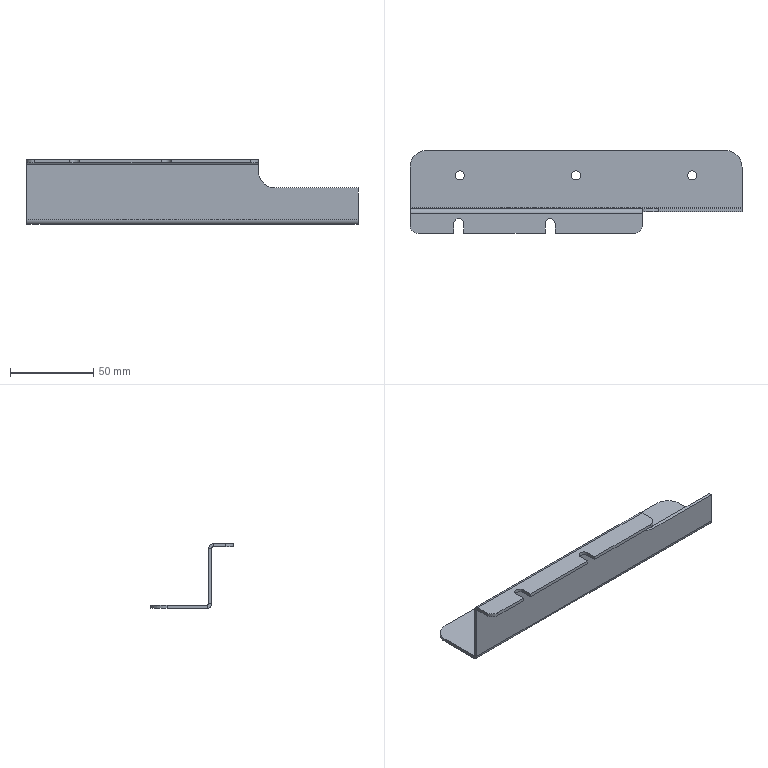Part | STEP file | 09-36 left support plate (Default) | 1 solid | 43 faces | box 200 x 50 x 39 mm | volume 30286 mm3 | plane 26 | cylinder 17 | commonest cylinder face diameters 5.5 x6 20 x3 1.473 x2 5.473 x2 6 x2 10 x2
STEP:
#1=CARTESIAN_POINT('',(-72.75,2.5,0.));
#2=VERTEX_POINT('',#1);
#3=CARTESIAN_POINT('',(-67.25,2.5,0.));
#4=VERTEX_POINT('',#3);
#5=CARTESIAN_POINT('',(-70.,2.5,0.));
#6=DIRECTION('',(0.,0.,1.));
#7=DIRECTION('',(1.,0.,0.));
#8=AXIS2_PLACEMENT_3D('',#5,#6,#7);
#9=CIRCLE('',#8,2.75);
#10=EDGE_CURVE('',#2,#4,#9,.T.);
#11=ORIENTED_EDGE('',*,*,#10,.T.);
#12=CARTESIAN_POINT('',(-67.25,2.5,-2.));
#13=VERTEX_POINT('',#12);
#14=CARTESIAN_POINT('',(-67.25,2.5,28.));
#15=DIRECTION('',(0.,0.,-1.));
#16=VECTOR('',#15,1000.);
#17=LINE('',#14,#16);
#18=EDGE_CURVE('',#4,#13,#17,.T.);
#19=ORIENTED_EDGE('',*,*,#18,.T.);
#20=CARTESIAN_POINT('',(-72.75,2.5,-2.));
#21=VERTEX_POINT('',#20);
#22=CARTESIAN_POINT('',(-70.,2.5,-2.));
#23=DIRECTION('',(0.,0.,-1.));
#24=DIRECTION('',(-1.,0.,0.));
#25=AXIS2_PLACEMENT_3D('',#22,#23,#24);
#26=CIRCLE('',#25,2.75);
#27=EDGE_CURVE('',#13,#21,#26,.T.);
#28=ORIENTED_EDGE('',*,*,#27,.T.);
#29=CARTESIAN_POINT('',(-72.75,2.5,28.));
#30=DIRECTION('',(0.,0.,-1.));
#31=VECTOR('',#30,1000.);
#32=LINE('',#29,#31);
#33=EDGE_CURVE('',#2,#21,#32,.T.);
#34=ORIENTED_EDGE('',*,*,#33,.F.);
#35=EDGE_LOOP('',(#11,#19,#28,#34));
#36=FACE_OUTER_BOUND('',#35,.T.);
#37=CARTESIAN_POINT('',(-70.,2.5,28.));
#38=DIRECTION('',(0.,0.,-1.));
#39=DIRECTION('',(-1.,0.,0.));
#40=AXIS2_PLACEMENT_3D('',#37,#38,#39);
#41=CYLINDRICAL_SURFACE('',#40,2.75);
#42=ADVANCED_FACE('',(#36),#41,.F.);
#43=CARTESIAN_POINT('',(-2.75,2.5,0.));
#44=VERTEX_POINT('',#43);
#45=CARTESIAN_POINT('',(2.75,2.5,0.));
#46=VERTEX_POINT('',#45);
#47=CARTESIAN_POINT('',(0.,2.5,0.));
#48=DIRECTION('',(0.,0.,1.));
#49=DIRECTION('',(1.,0.,0.));
#50=AXIS2_PLACEMENT_3D('',#47,#48,#49);
#51=CIRCLE('',#50,2.75);
#52=EDGE_CURVE('',#44,#46,#51,.T.);
#53=ORIENTED_EDGE('',*,*,#52,.T.);
#54=CARTESIAN_POINT('',(2.75,2.5,-2.));
#55=VERTEX_POINT('',#54);
#56=CARTESIAN_POINT('',(2.75,2.5,28.));
#57=DIRECTION('',(0.,0.,-1.));
#58=VECTOR('',#57,1000.);
#59=LINE('',#56,#58);
#60=EDGE_CURVE('',#46,#55,#59,.T.);
#61=ORIENTED_EDGE('',*,*,#60,.T.);
#62=CARTESIAN_POINT('',(-2.75,2.5,-2.));
#63=VERTEX_POINT('',#62);
#64=CARTESIAN_POINT('',(0.,2.5,-2.));
#65=DIRECTION('',(0.,0.,-1.));
#66=DIRECTION('',(-1.,0.,0.));
#67=AXIS2_PLACEMENT_3D('',#64,#65,#66);
#68=CIRCLE('',#67,2.75);
#69=EDGE_CURVE('',#55,#63,#68,.T.);
#70=ORIENTED_EDGE('',*,*,#69,.T.);
#71=CARTESIAN_POINT('',(-2.75,2.5,28.));
#72=DIRECTION('',(0.,0.,-1.));
#73=VECTOR('',#72,1000.);
#74=LINE('',#71,#73);
#75=EDGE_CURVE('',#44,#63,#74,.T.);
#76=ORIENTED_EDGE('',*,*,#75,.F.);
#77=EDGE_LOOP('',(#53,#61,#70,#76));
#78=FACE_OUTER_BOUND('',#77,.T.);
#79=CARTESIAN_POINT('',(0.,2.5,28.));
#80=DIRECTION('',(0.,0.,-1.));
#81=DIRECTION('',(-1.,0.,0.));
#82=AXIS2_PLACEMENT_3D('',#79,#80,#81);
#83=CYLINDRICAL_SURFACE('',#82,2.75);
#84=ADVANCED_FACE('',(#78),#83,.F.);
#85=CARTESIAN_POINT('',(67.25,2.5,0.));
#86=VERTEX_POINT('',#85);
#87=CARTESIAN_POINT('',(72.75,2.5,0.));
#88=VERTEX_POINT('',#87);
#89=CARTESIAN_POINT('',(70.,2.5,0.));
#90=DIRECTION('',(0.,0.,1.));
#91=DIRECTION('',(1.,0.,0.));
#92=AXIS2_PLACEMENT_3D('',#89,#90,#91);
#93=CIRCLE('',#92,2.75);
#94=EDGE_CURVE('',#86,#88,#93,.T.);
#95=ORIENTED_EDGE('',*,*,#94,.T.);
#96=CARTESIAN_POINT('',(72.75,2.5,-2.));
#97=VERTEX_POINT('',#96);
#98=CARTESIAN_POINT('',(72.75,2.5,28.));
#99=DIRECTION('',(0.,0.,-1.));
#100=VECTOR('',#99,1000.);
#101=LINE('',#98,#100);
#102=EDGE_CURVE('',#88,#97,#101,.T.);
#103=ORIENTED_EDGE('',*,*,#102,.T.);
#104=CARTESIAN_POINT('',(67.25,2.5,-2.));
#105=VERTEX_POINT('',#104);
#106=CARTESIAN_POINT('',(70.,2.5,-2.));
#107=DIRECTION('',(0.,0.,-1.));
#108=DIRECTION('',(-1.,0.,0.));
#109=AXIS2_PLACEMENT_3D('',#106,#107,#108);
#110=CIRCLE('',#109,2.75);
#111=EDGE_CURVE('',#97,#105,#110,.T.);
#112=ORIENTED_EDGE('',*,*,#111,.T.);
#113=CARTESIAN_POINT('',(67.25,2.5,28.));
#114=DIRECTION('',(0.,0.,-1.));
#115=VECTOR('',#114,1000.);
#116=LINE('',#113,#115);
#117=EDGE_CURVE('',#86,#105,#116,.T.);
#118=ORIENTED_EDGE('',*,*,#117,.F.);
#119=EDGE_LOOP('',(#95,#103,#112,#118));
#120=FACE_OUTER_BOUND('',#119,.T.);
#121=CARTESIAN_POINT('',(70.,2.5,28.));
#122=DIRECTION('',(0.,0.,-1.));
#123=DIRECTION('',(-1.,0.,0.));
#124=AXIS2_PLACEMENT_3D('',#121,#122,#123);
#125=CYLINDRICAL_SURFACE('',#124,2.75);
#126=ADVANCED_FACE('',(#120),#125,.F.);
#127=CARTESIAN_POINT('',(-12.6,-32.5,35.));
#128=VERTEX_POINT('',#127);
#129=CARTESIAN_POINT('',(-12.6,-32.5,37.));
#130=VERTEX_POINT('',#129);
#131=CARTESIAN_POINT('',(-12.6,-32.5,7.));
#132=DIRECTION('',(0.,0.,1.));
#133=VECTOR('',#132,1000.);
#134=LINE('',#131,#133);
#135=EDGE_CURVE('',#128,#130,#134,.T.);
#136=ORIENTED_EDGE('',*,*,#135,.F.);
#137=CARTESIAN_POINT('',(35.,-32.5,35.));
#138=VERTEX_POINT('',#137);
#139=CARTESIAN_POINT('',(-100.,-32.5,35.));
#140=DIRECTION('',(-1.,0.,0.));
#141=VECTOR('',#140,1000.);
#142=LINE('',#139,#141);
#143=EDGE_CURVE('',#138,#128,#142,.T.);
#144=ORIENTED_EDGE('',*,*,#143,.F.);
#145=CARTESIAN_POINT('',(35.,-32.5,37.));
#146=VERTEX_POINT('',#145);
#147=CARTESIAN_POINT('',(35.,-32.5,37.));
#148=DIRECTION('',(0.,0.,1.));
#149=VECTOR('',#148,1000.);
#150=LINE('',#147,#149);
#151=EDGE_CURVE('',#138,#146,#150,.T.);
#152=ORIENTED_EDGE('',*,*,#151,.T.);
#153=CARTESIAN_POINT('',(-100.,-32.5,37.));
#154=DIRECTION('',(-1.,0.,0.));
#155=VECTOR('',#154,1000.);
#156=LINE('',#153,#155);
#157=EDGE_CURVE('',#146,#130,#156,.T.);
#158=ORIENTED_EDGE('',*,*,#157,.T.);
#159=EDGE_LOOP('',(#136,#144,#152,#158));
#160=FACE_OUTER_BOUND('',#159,.T.);
#161=CARTESIAN_POINT('',(-100.,-32.5,37.));
#162=DIRECTION('',(0.,-1.,0.));
#163=DIRECTION('',(0.,0.,-1.));
#164=AXIS2_PLACEMENT_3D('',#161,#162,#163);
#165=PLANE('',#164);
#166=ADVANCED_FACE('',(#160),#165,.T.);
#167=CARTESIAN_POINT('',(-18.6,-32.5,35.));
#168=VERTEX_POINT('',#167);
#169=CARTESIAN_POINT('',(-18.6,-32.5,37.));
#170=VERTEX_POINT('',#169);
#171=CARTESIAN_POINT('',(-18.6,-32.5,7.));
#172=DIRECTION('',(0.,0.,1.));
#173=VECTOR('',#172,1000.);
#174=LINE('',#171,#173);
#175=EDGE_CURVE('',#168,#170,#174,.T.);
#176=ORIENTED_EDGE('',*,*,#175,.T.);
#177=CARTESIAN_POINT('',(-67.6,-32.5,37.));
#178=VERTEX_POINT('',#177);
#179=CARTESIAN_POINT('',(-100.,-32.5,37.));
#180=DIRECTION('',(-1.,0.,0.));
#181=VECTOR('',#180,1000.);
#182=LINE('',#179,#181);
#183=EDGE_CURVE('',#170,#178,#182,.T.);
#184=ORIENTED_EDGE('',*,*,#183,.T.);
#185=CARTESIAN_POINT('',(-67.6,-32.5,35.));
#186=VERTEX_POINT('',#185);
#187=CARTESIAN_POINT('',(-67.6,-32.5,7.));
#188=DIRECTION('',(0.,0.,1.));
#189=VECTOR('',#188,1000.);
#190=LINE('',#187,#189);
#191=EDGE_CURVE('',#186,#178,#190,.T.);
#192=ORIENTED_EDGE('',*,*,#191,.F.);
#193=CARTESIAN_POINT('',(-100.,-32.5,35.));
#194=DIRECTION('',(-1.,0.,0.));
#195=VECTOR('',#194,1000.);
#196=LINE('',#193,#195);
#197=EDGE_CURVE('',#168,#186,#196,.T.);
#198=ORIENTED_EDGE('',*,*,#197,.F.);
#199=EDGE_LOOP('',(#176,#184,#192,#198));
#200=FACE_OUTER_BOUND('',#199,.T.);
#201=CARTESIAN_POINT('',(-100.,-32.5,37.));
#202=DIRECTION('',(0.,-1.,0.));
#203=DIRECTION('',(0.,0.,-1.));
#204=AXIS2_PLACEMENT_3D('',#201,#202,#203);
#205=PLANE('',#204);
#206=ADVANCED_FACE('',(#200),#205,.T.);
#207=CARTESIAN_POINT('',(100.,-19.5,20.));
#208=VERTEX_POINT('',#207);
#209=CARTESIAN_POINT('',(100.,-19.5,0.7366));
#210=VERTEX_POINT('',#209);
#211=CARTESIAN_POINT('',(100.,-19.5,0.));
#212=DIRECTION('',(0.,0.,-1.));
#213=VECTOR('',#212,1000.);
#214=LINE('',#211,#213);
#215=EDGE_CURVE('',#208,#210,#214,.T.);
#216=ORIENTED_EDGE('',*,*,#215,.F.);
#217=CARTESIAN_POINT('',(50.,-19.5,20.));
#218=VERTEX_POINT('',#217);
#219=CARTESIAN_POINT('',(100.,-19.5,20.));
#220=DIRECTION('',(-1.,0.,0.));
#221=VECTOR('',#220,1000.);
#222=LINE('',#219,#221);
#223=EDGE_CURVE('',#208,#218,#222,.T.);
#224=ORIENTED_EDGE('',*,*,#223,.T.);
#225=CARTESIAN_POINT('',(40.,-19.5,30.));
#226=VERTEX_POINT('',#225);
#227=CARTESIAN_POINT('',(50.,-19.5,30.));
#228=DIRECTION('',(0.,1.,0.));
#229=DIRECTION('',(0.,0.,1.));
#230=AXIS2_PLACEMENT_3D('',#227,#228,#229);
#231=CIRCLE('',#230,10.);
#232=EDGE_CURVE('',#218,#226,#231,.T.);
#233=ORIENTED_EDGE('',*,*,#232,.T.);
#234=CARTESIAN_POINT('',(40.,-19.5,34.263));
#235=VERTEX_POINT('',#234);
#236=CARTESIAN_POINT('',(40.,-19.5,0.));
#237=DIRECTION('',(0.,0.,1.));
#238=VECTOR('',#237,1000.);
#239=LINE('',#236,#238);
#240=EDGE_CURVE('',#226,#235,#239,.T.);
#241=ORIENTED_EDGE('',*,*,#240,.T.);
#242=CARTESIAN_POINT('',(-100.,-19.5,34.263));
#243=VERTEX_POINT('',#242);
#244=CARTESIAN_POINT('',(-100.,-19.5,34.263));
#245=DIRECTION('',(1.,0.,0.));
#246=VECTOR('',#245,1000.);
#247=LINE('',#244,#246);
#248=EDGE_CURVE('',#243,#235,#247,.T.);
#249=ORIENTED_EDGE('',*,*,#248,.F.);
#250=CARTESIAN_POINT('',(-100.,-19.5,0.7366));
#251=VERTEX_POINT('',#250);
#252=CARTESIAN_POINT('',(-100.,-19.5,35.));
#253=DIRECTION('',(0.,0.,1.));
#254=VECTOR('',#253,1000.);
#255=LINE('',#252,#254);
#256=EDGE_CURVE('',#251,#243,#255,.T.);
#257=ORIENTED_EDGE('',*,*,#256,.F.);
#258=CARTESIAN_POINT('',(100.,-19.5,0.7366));
#259=DIRECTION('',(1.,0.,0.));
#260=VECTOR('',#259,1000.);
#261=LINE('',#258,#260);
#262=EDGE_CURVE('',#251,#210,#261,.T.);
#263=ORIENTED_EDGE('',*,*,#262,.T.);
#264=EDGE_LOOP('',(#216,#224,#233,#241,#249,#257,#263));
#265=FACE_OUTER_BOUND('',#264,.T.);
#266=CARTESIAN_POINT('',(100.,-19.5,0.));
#267=DIRECTION('',(0.,-1.,0.));
#268=DIRECTION('',(0.,0.,-1.));
#269=AXIS2_PLACEMENT_3D('',#266,#267,#268);
#270=PLANE('',#269);
#271=ADVANCED_FACE('',(#265),#270,.T.);
#272=CARTESIAN_POINT('',(100.,-17.5,20.));
#273=VERTEX_POINT('',#272);
#274=CARTESIAN_POINT('',(50.,-17.5,20.));
#275=VERTEX_POINT('',#274);
#276=CARTESIAN_POINT('',(126.294,-17.5,20.));
#277=DIRECTION('',(-1.,0.,0.));
#278=VECTOR('',#277,1000.);
#279=LINE('',#276,#278);
#280=EDGE_CURVE('',#273,#275,#279,.T.);
#281=ORIENTED_EDGE('',*,*,#280,.F.);
#282=CARTESIAN_POINT('',(100.,-17.5,0.7366));
#283=VERTEX_POINT('',#282);
#284=CARTESIAN_POINT('',(100.,-17.5,0.));
#285=DIRECTION('',(0.,0.,-1.));
#286=VECTOR('',#285,1000.);
#287=LINE('',#284,#286);
#288=EDGE_CURVE('',#273,#283,#287,.T.);
#289=ORIENTED_EDGE('',*,*,#288,.T.);
#290=CARTESIAN_POINT('',(-100.,-17.5,0.7366));
#291=VERTEX_POINT('',#290);
#292=CARTESIAN_POINT('',(-100.,-17.5,0.7366));
#293=DIRECTION('',(1.,0.,0.));
#294=VECTOR('',#293,1000.);
#295=LINE('',#292,#294);
#296=EDGE_CURVE('',#291,#283,#295,.T.);
#297=ORIENTED_EDGE('',*,*,#296,.F.);
#298=CARTESIAN_POINT('',(-100.,-17.5,34.263));
#299=VERTEX_POINT('',#298);
#300=CARTESIAN_POINT('',(-100.,-17.5,35.));
#301=DIRECTION('',(0.,0.,1.));
#302=VECTOR('',#301,1000.);
#303=LINE('',#300,#302);
#304=EDGE_CURVE('',#291,#299,#303,.T.);
#305=ORIENTED_EDGE('',*,*,#304,.T.);
#306=CARTESIAN_POINT('',(40.,-17.5,34.263));
#307=VERTEX_POINT('',#306);
#308=CARTESIAN_POINT('',(-100.,-17.5,34.263));
#309=DIRECTION('',(1.,0.,0.));
#310=VECTOR('',#309,1000.);
#311=LINE('',#308,#310);
#312=EDGE_CURVE('',#299,#307,#311,.T.);
#313=ORIENTED_EDGE('',*,*,#312,.T.);
#314=CARTESIAN_POINT('',(40.,-17.5,30.));
#315=VERTEX_POINT('',#314);
#316=CARTESIAN_POINT('',(40.,-17.5,30.));
#317=DIRECTION('',(0.,0.,1.));
#318=VECTOR('',#317,1000.);
#319=LINE('',#316,#318);
#320=EDGE_CURVE('',#315,#307,#319,.T.);
#321=ORIENTED_EDGE('',*,*,#320,.F.);
#322=CARTESIAN_POINT('',(50.,-17.5,30.));
#323=DIRECTION('',(0.,1.,0.));
#324=DIRECTION('',(0.,0.,-1.));
#325=AXIS2_PLACEMENT_3D('',#322,#323,#324);
#326=CIRCLE('',#325,10.);
#327=EDGE_CURVE('',#275,#315,#326,.T.);
#328=ORIENTED_EDGE('',*,*,#327,.F.);
#329=EDGE_LOOP('',(#281,#289,#297,#305,#313,#321,#328));
#330=FACE_OUTER_BOUND('',#329,.T.);
#331=CARTESIAN_POINT('',(100.,-17.5,0.));
#332=DIRECTION('',(0.,-1.,0.));
#333=DIRECTION('',(0.,0.,-1.));
#334=AXIS2_PLACEMENT_3D('',#331,#332,#333);
#335=PLANE('',#334);
#336=ADVANCED_FACE('',(#330),#335,.F.);
#337=ORIENTED_EDGE('',*,*,#288,.F.);
#338=CARTESIAN_POINT('',(100.,-17.5,20.));
#339=DIRECTION('',(0.,-1.,0.));
#340=VECTOR('',#339,1000.);
#341=LINE('',#338,#340);
#342=EDGE_CURVE('',#273,#208,#341,.T.);
#343=ORIENTED_EDGE('',*,*,#342,.T.);
#344=ORIENTED_EDGE('',*,*,#215,.T.);
#345=CARTESIAN_POINT('',(100.,-17.5,0.7366));
#346=DIRECTION('',(0.,-1.,0.));
#347=VECTOR('',#346,1000.);
#348=LINE('',#345,#347);
#349=EDGE_CURVE('',#283,#210,#348,.T.);
#350=ORIENTED_EDGE('',*,*,#349,.F.);
#351=EDGE_LOOP('',(#337,#343,#344,#350));
#352=FACE_OUTER_BOUND('',#351,.T.);
#353=CARTESIAN_POINT('',(100.,-19.5,0.));
#354=DIRECTION('',(1.,0.,0.));
#355=DIRECTION('',(0.,0.,-1.));
#356=AXIS2_PLACEMENT_3D('',#353,#354,#355);
#357=PLANE('',#356);
#358=ADVANCED_FACE('',(#352),#357,.T.);
#359=CARTESIAN_POINT('',(40.,-20.237,37.));
#360=VERTEX_POINT('',#359);
#361=CARTESIAN_POINT('',(-100.,-20.237,37.));
#362=VERTEX_POINT('',#361);
#363=CARTESIAN_POINT('',(-100.,-20.237,37.));
#364=DIRECTION('',(-1.,0.,0.));
#365=VECTOR('',#364,1000.);
#366=LINE('',#363,#365);
#367=EDGE_CURVE('',#360,#362,#366,.T.);
#368=ORIENTED_EDGE('',*,*,#367,.F.);
#369=CARTESIAN_POINT('',(40.,-20.237,34.263));
#370=DIRECTION('',(1.,0.,0.));
#371=DIRECTION('',(0.,0.,1.));
#372=AXIS2_PLACEMENT_3D('',#369,#370,#371);
#373=CIRCLE('',#372,2.737);
#374=EDGE_CURVE('',#307,#360,#373,.T.);
#375=ORIENTED_EDGE('',*,*,#374,.F.);
#376=ORIENTED_EDGE('',*,*,#312,.F.);
#377=CARTESIAN_POINT('',(-100.,-20.237,34.263));
#378=DIRECTION('',(-1.,0.,0.));
#379=DIRECTION('',(0.,0.,1.));
#380=AXIS2_PLACEMENT_3D('',#377,#378,#379);
#381=CIRCLE('',#380,2.737);
#382=EDGE_CURVE('',#362,#299,#381,.T.);
#383=ORIENTED_EDGE('',*,*,#382,.F.);
#384=EDGE_LOOP('',(#368,#375,#376,#383));
#385=FACE_OUTER_BOUND('',#384,.T.);
#386=CARTESIAN_POINT('',(-100.,-20.237,34.263));
#387=DIRECTION('',(-1.,0.,0.));
#388=DIRECTION('',(0.,0.,1.));
#389=AXIS2_PLACEMENT_3D('',#386,#387,#388);
#390=CYLINDRICAL_SURFACE('',#389,2.737);
#391=ADVANCED_FACE('',(#385),#390,.T.);
#392=CARTESIAN_POINT('',(40.,-20.237,35.));
#393=VERTEX_POINT('',#392);
#394=CARTESIAN_POINT('',(40.,-20.237,34.263));
#395=DIRECTION('',(1.,0.,0.));
#396=DIRECTION('',(0.,0.,1.));
#397=AXIS2_PLACEMENT_3D('',#394,#395,#396);
#398=CIRCLE('',#397,0.7366);
#399=EDGE_CURVE('',#235,#393,#398,.T.);
#400=ORIENTED_EDGE('',*,*,#399,.T.);
#401=CARTESIAN_POINT('',(-100.,-20.237,35.));
#402=VERTEX_POINT('',#401);
#403=CARTESIAN_POINT('',(100.,-20.237,35.));
#404=DIRECTION('',(-1.,0.,0.));
#405=VECTOR('',#404,1000.);
#406=LINE('',#403,#405);
#407=EDGE_CURVE('',#393,#402,#406,.T.);
#408=ORIENTED_EDGE('',*,*,#407,.T.);
#409=CARTESIAN_POINT('',(-100.,-20.237,34.263));
#410=DIRECTION('',(-1.,0.,0.));
#411=DIRECTION('',(0.,0.,1.));
#412=AXIS2_PLACEMENT_3D('',#409,#410,#411);
#413=CIRCLE('',#412,0.7366);
#414=EDGE_CURVE('',#402,#243,#413,.T.);
#415=ORIENTED_EDGE('',*,*,#414,.T.);
#416=ORIENTED_EDGE('',*,*,#248,.T.);
#417=EDGE_LOOP('',(#400,#408,#415,#416));
#418=FACE_OUTER_BOUND('',#417,.T.);
#419=CARTESIAN_POINT('',(-100.,-20.237,34.263));
#420=DIRECTION('',(-1.,0.,0.));
#421=DIRECTION('',(0.,0.,1.));
#422=AXIS2_PLACEMENT_3D('',#419,#420,#421);
#423=CYLINDRICAL_SURFACE('',#422,0.7366);
#424=ADVANCED_FACE('',(#418),#423,.F.);
#425=CARTESIAN_POINT('',(-12.6,-26.5,37.));
#426=VERTEX_POINT('',#425);
#427=CARTESIAN_POINT('',(-12.6,-26.5,37.));
#428=DIRECTION('',(0.,1.,0.));
#429=VECTOR('',#428,1000.);
#430=LINE('',#427,#429);
#431=EDGE_CURVE('',#130,#426,#430,.T.);
#432=ORIENTED_EDGE('',*,*,#431,.F.);
#433=ORIENTED_EDGE('',*,*,#157,.F.);
#434=CARTESIAN_POINT('',(40.,-27.5,37.));
#435=VERTEX_POINT('',#434);
#436=CARTESIAN_POINT('',(35.,-27.5,37.));
#437=DIRECTION('',(0.,0.,1.));
#438=DIRECTION('',(1.,0.,0.));
#439=AXIS2_PLACEMENT_3D('',#436,#437,#438);
#440=CIRCLE('',#439,5.);
#441=EDGE_CURVE('',#146,#435,#440,.T.);
#442=ORIENTED_EDGE('',*,*,#441,.T.);
#443=CARTESIAN_POINT('',(40.,-19.5,37.));
#444=DIRECTION('',(0.,-1.,0.));
#445=VECTOR('',#444,1000.);
#446=LINE('',#443,#445);
#447=EDGE_CURVE('',#360,#435,#446,.T.);
#448=ORIENTED_EDGE('',*,*,#447,.F.);
#449=ORIENTED_EDGE('',*,*,#367,.T.);
#450=CARTESIAN_POINT('',(-100.,-27.5,37.));
#451=VERTEX_POINT('',#450);
#452=CARTESIAN_POINT('',(-100.,-19.5,37.));
#453=DIRECTION('',(0.,1.,0.));
#454=VECTOR('',#453,1000.);
#455=LINE('',#452,#454);
#456=EDGE_CURVE('',#451,#362,#455,.T.);
#457=ORIENTED_EDGE('',*,*,#456,.F.);
#458=CARTESIAN_POINT('',(-95.,-32.5,37.));
#459=VERTEX_POINT('',#458);
#460=CARTESIAN_POINT('',(-95.,-27.5,37.));
#461=DIRECTION('',(0.,0.,1.));
#462=DIRECTION('',(1.,0.,0.));
#463=AXIS2_PLACEMENT_3D('',#460,#461,#462);
#464=CIRCLE('',#463,5.);
#465=EDGE_CURVE('',#451,#459,#464,.T.);
#466=ORIENTED_EDGE('',*,*,#465,.T.);
#467=CARTESIAN_POINT('',(-73.6,-32.5,37.));
#468=VERTEX_POINT('',#467);
#469=CARTESIAN_POINT('',(-100.,-32.5,37.));
#470=DIRECTION('',(-1.,0.,0.));
#471=VECTOR('',#470,1000.);
#472=LINE('',#469,#471);
#473=EDGE_CURVE('',#468,#459,#472,.T.);
#474=ORIENTED_EDGE('',*,*,#473,.F.);
#475=CARTESIAN_POINT('',(-73.6,-26.5,37.));
#476=VERTEX_POINT('',#475);
#477=CARTESIAN_POINT('',(-73.6,-26.5,37.));
#478=DIRECTION('',(0.,-1.,0.));
#479=VECTOR('',#478,1000.);
#480=LINE('',#477,#479);
#481=EDGE_CURVE('',#476,#468,#480,.T.);
#482=ORIENTED_EDGE('',*,*,#481,.F.);
#483=CARTESIAN_POINT('',(-67.6,-26.5,37.));
#484=VERTEX_POINT('',#483);
#485=CARTESIAN_POINT('',(-70.6,-26.5,37.));
#486=DIRECTION('',(0.,0.,1.));
#487=DIRECTION('',(1.,0.,0.));
#488=AXIS2_PLACEMENT_3D('',#485,#486,#487);
#489=CIRCLE('',#488,3.);
#490=EDGE_CURVE('',#484,#476,#489,.T.);
#491=ORIENTED_EDGE('',*,*,#490,.F.);
#492=CARTESIAN_POINT('',(-67.6,-26.5,37.));
#493=DIRECTION('',(0.,1.,0.));
#494=VECTOR('',#493,1000.);
#495=LINE('',#492,#494);
#496=EDGE_CURVE('',#178,#484,#495,.T.);
#497=ORIENTED_EDGE('',*,*,#496,.F.);
#498=ORIENTED_EDGE('',*,*,#183,.F.);
#499=CARTESIAN_POINT('',(-18.6,-26.5,37.));
#500=VERTEX_POINT('',#499);
#501=CARTESIAN_POINT('',(-18.6,-26.5,37.));
#502=DIRECTION('',(0.,-1.,0.));
#503=VECTOR('',#502,1000.);
#504=LINE('',#501,#503);
#505=EDGE_CURVE('',#500,#170,#504,.T.);
#506=ORIENTED_EDGE('',*,*,#505,.F.);
#507=CARTESIAN_POINT('',(-15.6,-26.5,37.));
#508=DIRECTION('',(0.,0.,1.));
#509=DIRECTION('',(1.,0.,0.));
#510=AXIS2_PLACEMENT_3D('',#507,#508,#509);
#511=CIRCLE('',#510,3.);
#512=EDGE_CURVE('',#426,#500,#511,.T.);
#513=ORIENTED_EDGE('',*,*,#512,.F.);
#514=EDGE_LOOP('',(#432,#433,#442,#448,#449,#457,#466,#474,#482,#491,#497,#498,#506,#513));
#515=FACE_OUTER_BOUND('',#514,.T.);
#516=CARTESIAN_POINT('',(-100.,-19.5,37.));
#517=DIRECTION('',(0.,0.,1.));
#518=DIRECTION('',(1.,0.,0.));
#519=AXIS2_PLACEMENT_3D('',#516,#517,#518);
#520=PLANE('',#519);
#521=ADVANCED_FACE('',(#515),#520,.T.);
#522=ORIENTED_EDGE('',*,*,#143,.T.);
#523=CARTESIAN_POINT('',(-12.6,-26.5,35.));
#524=VERTEX_POINT('',#523);
#525=CARTESIAN_POINT('',(-12.6,-19.5,35.));
#526=DIRECTION('',(0.,1.,0.));
#527=VECTOR('',#526,1000.);
#528=LINE('',#525,#527);
#529=EDGE_CURVE('',#128,#524,#528,.T.);
#530=ORIENTED_EDGE('',*,*,#529,.T.);
#531=CARTESIAN_POINT('',(-18.6,-26.5,35.));
#532=VERTEX_POINT('',#531);
#533=CARTESIAN_POINT('',(-15.6,-26.5,35.));
#534=DIRECTION('',(0.,0.,1.));
#535=DIRECTION('',(1.,0.,0.));
#536=AXIS2_PLACEMENT_3D('',#533,#534,#535);
#537=CIRCLE('',#536,3.);
#538=EDGE_CURVE('',#524,#532,#537,.T.);
#539=ORIENTED_EDGE('',*,*,#538,.T.);
#540=CARTESIAN_POINT('',(-18.6,-19.5,35.));
#541=DIRECTION('',(0.,-1.,0.));
#542=VECTOR('',#541,1000.);
#543=LINE('',#540,#542);
#544=EDGE_CURVE('',#532,#168,#543,.T.);
#545=ORIENTED_EDGE('',*,*,#544,.T.);
#546=ORIENTED_EDGE('',*,*,#197,.T.);
#547=CARTESIAN_POINT('',(-67.6,-26.5,35.));
#548=VERTEX_POINT('',#547);
#549=CARTESIAN_POINT('',(-67.6,-19.5,35.));
#550=DIRECTION('',(0.,1.,0.));
#551=VECTOR('',#550,1000.);
#552=LINE('',#549,#551);
#553=EDGE_CURVE('',#186,#548,#552,.T.);
#554=ORIENTED_EDGE('',*,*,#553,.T.);
#555=CARTESIAN_POINT('',(-73.6,-26.5,35.));
#556=VERTEX_POINT('',#555);
#557=CARTESIAN_POINT('',(-70.6,-26.5,35.));
#558=DIRECTION('',(0.,0.,1.));
#559=DIRECTION('',(1.,0.,0.));
#560=AXIS2_PLACEMENT_3D('',#557,#558,#559);
#561=CIRCLE('',#560,3.);
#562=EDGE_CURVE('',#548,#556,#561,.T.);
#563=ORIENTED_EDGE('',*,*,#562,.T.);
#564=CARTESIAN_POINT('',(-73.6,-32.5,35.));
#565=VERTEX_POINT('',#564);
#566=CARTESIAN_POINT('',(-73.6,-19.5,35.));
#567=DIRECTION('',(0.,-1.,0.));
#568=VECTOR('',#567,1000.);
#569=LINE('',#566,#568);
#570=EDGE_CURVE('',#556,#565,#569,.T.);
#571=ORIENTED_EDGE('',*,*,#570,.T.);
#572=CARTESIAN_POINT('',(-95.,-32.5,35.));
#573=VERTEX_POINT('',#572);
#574=CARTESIAN_POINT('',(-100.,-32.5,35.));
#575=DIRECTION('',(-1.,0.,0.));
#576=VECTOR('',#575,1000.);
#577=LINE('',#574,#576);
#578=EDGE_CURVE('',#565,#573,#577,.T.);
#579=ORIENTED_EDGE('',*,*,#578,.T.);
#580=CARTESIAN_POINT('',(-100.,-27.5,35.));
#581=VERTEX_POINT('',#580);
#582=CARTESIAN_POINT('',(-95.,-27.5,35.));
#583=DIRECTION('',(0.,0.,-1.));
#584=DIRECTION('',(1.,0.,0.));
#585=AXIS2_PLACEMENT_3D('',#582,#583,#584);
#586=CIRCLE('',#585,5.);
#587=EDGE_CURVE('',#573,#581,#586,.T.);
#588=ORIENTED_EDGE('',*,*,#587,.T.);
#589=CARTESIAN_POINT('',(-100.,-19.5,35.));
#590=DIRECTION('',(0.,1.,0.));
#591=VECTOR('',#590,1000.);
#592=LINE('',#589,#591);
#593=EDGE_CURVE('',#581,#402,#592,.T.);
#594=ORIENTED_EDGE('',*,*,#593,.T.);
#595=ORIENTED_EDGE('',*,*,#407,.F.);
#596=CARTESIAN_POINT('',(40.,-27.5,35.));
#597=VERTEX_POINT('',#596);
#598=CARTESIAN_POINT('',(40.,-19.5,35.));
#599=DIRECTION('',(0.,-1.,0.));
#600=VECTOR('',#599,1000.);
#601=LINE('',#598,#600);
#602=EDGE_CURVE('',#393,#597,#601,.T.);
#603=ORIENTED_EDGE('',*,*,#602,.T.);
#604=CARTESIAN_POINT('',(35.,-27.5,35.));
#605=DIRECTION('',(0.,0.,-1.));
#606=DIRECTION('',(1.,0.,0.));
#607=AXIS2_PLACEMENT_3D('',#604,#605,#606);
#608=CIRCLE('',#607,5.);
#609=EDGE_CURVE('',#597,#138,#608,.T.);
#610=ORIENTED_EDGE('',*,*,#609,.T.);
#611=EDGE_LOOP('',(#522,#530,#539,#545,#546,#554,#563,#571,#579,#588,#594,#595,#603,#610));
#612=FACE_OUTER_BOUND('',#611,.T.);
#613=CARTESIAN_POINT('',(-100.,-19.5,35.));
#614=DIRECTION('',(0.,0.,1.));
#615=DIRECTION('',(1.,0.,0.));
#616=AXIS2_PLACEMENT_3D('',#613,#614,#615);
#617=PLANE('',#616);
#618=ADVANCED_FACE('',(#612),#617,.F.);
#619=CARTESIAN_POINT('',(-73.6,-32.5,37.));
#620=DIRECTION('',(0.,0.,-1.));
#621=VECTOR('',#620,1000.);
#622=LINE('',#619,#621);
#623=EDGE_CURVE('',#468,#565,#622,.T.);
#624=ORIENTED_EDGE('',*,*,#623,.F.);
#625=ORIENTED_EDGE('',*,*,#473,.T.);
#626=CARTESIAN_POINT('',(-95.,-32.5,37.));
#627=DIRECTION('',(0.,0.,-1.));
#628=VECTOR('',#627,1000.);
#629=LINE('',#626,#628);
#630=EDGE_CURVE('',#459,#573,#629,.T.);
#631=ORIENTED_EDGE('',*,*,#630,.T.);
#632=ORIENTED_EDGE('',*,*,#578,.F.);
#633=EDGE_LOOP('',(#624,#625,#631,#632));
#634=FACE_OUTER_BOUND('',#633,.T.);
#635=CARTESIAN_POINT('',(-100.,-32.5,37.));
#636=DIRECTION('',(0.,-1.,0.));
#637=DIRECTION('',(0.,0.,-1.));
#638=AXIS2_PLACEMENT_3D('',#635,#636,#637);
#639=PLANE('',#638);
#640=ADVANCED_FACE('',(#634),#639,.T.);
#641=ORIENTED_EDGE('',*,*,#256,.T.);
#642=CARTESIAN_POINT('',(-100.,-19.5,34.263));
#643=DIRECTION('',(0.,1.,0.));
#644=VECTOR('',#643,1000.);
#645=LINE('',#642,#644);
#646=EDGE_CURVE('',#243,#299,#645,.T.);
#647=ORIENTED_EDGE('',*,*,#646,.T.);
#648=ORIENTED_EDGE('',*,*,#304,.F.);
#649=CARTESIAN_POINT('',(-100.,-17.5,0.7366));
#650=DIRECTION('',(0.,-1.,0.));
#651=VECTOR('',#650,1000.);
#652=LINE('',#649,#651);
#653=EDGE_CURVE('',#291,#251,#652,.T.);
#654=ORIENTED_EDGE('',*,*,#653,.T.);
#655=EDGE_LOOP('',(#641,#647,#648,#654));
#656=FACE_OUTER_BOUND('',#655,.T.);
#657=CARTESIAN_POINT('',(-100.,-19.5,35.));
#658=DIRECTION('',(-1.,0.,0.));
#659=DIRECTION('',(0.,0.,1.));
#660=AXIS2_PLACEMENT_3D('',#657,#658,#659);
#661=PLANE('',#660);
#662=ADVANCED_FACE('',(#656),#661,.T.);
#663=CARTESIAN_POINT('',(100.,-16.763,-2.));
#664=VERTEX_POINT('',#663);
#665=CARTESIAN_POINT('',(100.,7.5,-2.));
#666=VERTEX_POINT('',#665);
#667=CARTESIAN_POINT('',(100.,17.5,-2.));
#668=DIRECTION('',(0.,1.,0.));
#669=VECTOR('',#668,1000.);
#670=LINE('',#667,#669);
#671=EDGE_CURVE('',#664,#666,#670,.T.);
#672=ORIENTED_EDGE('',*,*,#671,.T.);
#673=CARTESIAN_POINT('',(100.,7.5,0.));
#674=VERTEX_POINT('',#673);
#675=CARTESIAN_POINT('',(100.,7.5,-2.));
#676=DIRECTION('',(0.,0.,1.));
#677=VECTOR('',#676,1000.);
#678=LINE('',#675,#677);
#679=EDGE_CURVE('',#666,#674,#678,.T.);
#680=ORIENTED_EDGE('',*,*,#679,.T.);
#681=CARTESIAN_POINT('',(100.,-16.763,0.));
#682=VERTEX_POINT('',#681);
#683=CARTESIAN_POINT('',(100.,17.5,0.));
#684=DIRECTION('',(0.,1.,0.));
#685=VECTOR('',#684,1000.);
#686=LINE('',#683,#685);
#687=EDGE_CURVE('',#682,#674,#686,.T.);
#688=ORIENTED_EDGE('',*,*,#687,.F.);
#689=CARTESIAN_POINT('',(100.,-16.763,0.));
#690=DIRECTION('',(0.,0.,-1.));
#691=VECTOR('',#690,1000.);
#692=LINE('',#689,#691);
#693=EDGE_CURVE('',#682,#664,#692,.T.);
#694=ORIENTED_EDGE('',*,*,#693,.T.);
#695=EDGE_LOOP('',(#672,#680,#688,#694));
#696=FACE_OUTER_BOUND('',#695,.T.);
#697=CARTESIAN_POINT('',(100.,17.5,-2.));
#698=DIRECTION('',(1.,0.,0.));
#699=DIRECTION('',(0.,0.,-1.));
#700=AXIS2_PLACEMENT_3D('',#697,#698,#699);
#701=PLANE('',#700);
#702=ADVANCED_FACE('',(#696),#701,.T.);
#703=CARTESIAN_POINT('',(0.,2.5,-2.));
#704=DIRECTION('',(0.,0.,-1.));
#705=DIRECTION('',(-1.,0.,0.));
#706=AXIS2_PLACEMENT_3D('',#703,#704,#705);
#707=CIRCLE('',#706,2.75);
#708=EDGE_CURVE('',#63,#55,#707,.T.);
#709=ORIENTED_EDGE('',*,*,#708,.F.);
#710=ORIENTED_EDGE('',*,*,#69,.F.);
#711=EDGE_LOOP('',(#709,#710));
#712=FACE_BOUND('',#711,.T.);
#713=CARTESIAN_POINT('',(70.,2.5,-2.));
#714=DIRECTION('',(0.,0.,-1.));
#715=DIRECTION('',(-1.,0.,0.));
#716=AXIS2_PLACEMENT_3D('',#713,#714,#715);
#717=CIRCLE('',#716,2.75);
#718=EDGE_CURVE('',#105,#97,#717,.T.);
#719=ORIENTED_EDGE('',*,*,#718,.F.);
#720=ORIENTED_EDGE('',*,*,#111,.F.);
#721=EDGE_LOOP('',(#719,#720));
#722=FACE_BOUND('',#721,.T.);
#723=CARTESIAN_POINT('',(90.,17.5,-2.));
#724=VERTEX_POINT('',#723);
#725=CARTESIAN_POINT('',(-90.,17.5,-2.));
#726=VERTEX_POINT('',#725);
#727=CARTESIAN_POINT('',(-100.,17.5,-2.));
#728=DIRECTION('',(-1.,0.,0.));
#729=VECTOR('',#728,1000.);
#730=LINE('',#727,#729);
#731=EDGE_CURVE('',#724,#726,#730,.T.);
#732=ORIENTED_EDGE('',*,*,#731,.F.);
#733=CARTESIAN_POINT('',(90.,7.5,-2.));
#734=DIRECTION('',(0.,0.,-1.));
#735=DIRECTION('',(1.,0.,0.));
#736=AXIS2_PLACEMENT_3D('',#733,#734,#735);
#737=CIRCLE('',#736,10.);
#738=EDGE_CURVE('',#724,#666,#737,.T.);
#739=ORIENTED_EDGE('',*,*,#738,.T.);
#740=ORIENTED_EDGE('',*,*,#671,.F.);
#741=CARTESIAN_POINT('',(-100.,-16.763,-2.));
#742=VERTEX_POINT('',#741);
#743=CARTESIAN_POINT('',(100.,-16.763,-2.));
#744=DIRECTION('',(-1.,0.,0.));
#745=VECTOR('',#744,1000.);
#746=LINE('',#743,#745);
#747=EDGE_CURVE('',#664,#742,#746,.T.);
#748=ORIENTED_EDGE('',*,*,#747,.T.);
#749=CARTESIAN_POINT('',(-100.,7.5,-2.));
#750=VERTEX_POINT('',#749);
#751=CARTESIAN_POINT('',(-100.,17.5,-2.));
#752=DIRECTION('',(0.,-1.,0.));
#753=VECTOR('',#752,1000.);
#754=LINE('',#751,#753);
#755=EDGE_CURVE('',#750,#742,#754,.T.);
#756=ORIENTED_EDGE('',*,*,#755,.F.);
#757=CARTESIAN_POINT('',(-90.,7.5,-2.));
#758=DIRECTION('',(0.,0.,-1.));
#759=DIRECTION('',(1.,0.,0.));
#760=AXIS2_PLACEMENT_3D('',#757,#758,#759);
#761=CIRCLE('',#760,10.);
#762=EDGE_CURVE('',#750,#726,#761,.T.);
#763=ORIENTED_EDGE('',*,*,#762,.T.);
#764=EDGE_LOOP('',(#732,#739,#740,#748,#756,#763));
#765=FACE_OUTER_BOUND('',#764,.T.);
#766=CARTESIAN_POINT('',(-70.,2.5,-2.));
#767=DIRECTION('',(0.,0.,-1.));
#768=DIRECTION('',(-1.,0.,0.));
#769=AXIS2_PLACEMENT_3D('',#766,#767,#768);
#770=CIRCLE('',#769,2.75);
#771=EDGE_CURVE('',#21,#13,#770,.T.);
#772=ORIENTED_EDGE('',*,*,#771,.F.);
#773=ORIENTED_EDGE('',*,*,#27,.F.);
#774=EDGE_LOOP('',(#772,#773));
#775=FACE_BOUND('',#774,.T.);
#776=CARTESIAN_POINT('',(100.,-17.5,-2.));
#777=DIRECTION('',(0.,0.,1.));
#778=DIRECTION('',(1.,0.,0.));
#779=AXIS2_PLACEMENT_3D('',#776,#777,#778);
#780=PLANE('',#779);
#781=ADVANCED_FACE('',(#712,#722,#765,#775),#780,.F.);
#782=ORIENTED_EDGE('',*,*,#52,.F.);
#783=CARTESIAN_POINT('',(0.,2.5,0.));
#784=DIRECTION('',(0.,0.,1.));
#785=DIRECTION('',(1.,0.,0.));
#786=AXIS2_PLACEMENT_3D('',#783,#784,#785);
#787=CIRCLE('',#786,2.75);
#788=EDGE_CURVE('',#46,#44,#787,.T.);
#789=ORIENTED_EDGE('',*,*,#788,.F.);
#790=EDGE_LOOP('',(#782,#789));
#791=FACE_BOUND('',#790,.T.);
#792=ORIENTED_EDGE('',*,*,#94,.F.);
#793=CARTESIAN_POINT('',(70.,2.5,0.));
#794=DIRECTION('',(0.,0.,1.));
#795=DIRECTION('',(1.,0.,0.));
#796=AXIS2_PLACEMENT_3D('',#793,#794,#795);
#797=CIRCLE('',#796,2.75);
#798=EDGE_CURVE('',#88,#86,#797,.T.);
#799=ORIENTED_EDGE('',*,*,#798,.F.);
#800=EDGE_LOOP('',(#792,#799));
#801=FACE_BOUND('',#800,.T.);
#802=ORIENTED_EDGE('',*,*,#687,.T.);
#803=CARTESIAN_POINT('',(90.,17.5,0.));
#804=VERTEX_POINT('',#803);
#805=CARTESIAN_POINT('',(90.,7.5,0.));
#806=DIRECTION('',(0.,0.,1.));
#807=DIRECTION('',(1.,0.,0.));
#808=AXIS2_PLACEMENT_3D('',#805,#806,#807);
#809=CIRCLE('',#808,10.);
#810=EDGE_CURVE('',#674,#804,#809,.T.);
#811=ORIENTED_EDGE('',*,*,#810,.T.);
#812=CARTESIAN_POINT('',(-90.,17.5,0.));
#813=VERTEX_POINT('',#812);
#814=CARTESIAN_POINT('',(-100.,17.5,0.));
#815=DIRECTION('',(-1.,0.,0.));
#816=VECTOR('',#815,1000.);
#817=LINE('',#814,#816);
#818=EDGE_CURVE('',#804,#813,#817,.T.);
#819=ORIENTED_EDGE('',*,*,#818,.T.);
#820=CARTESIAN_POINT('',(-100.,7.5,0.));
#821=VERTEX_POINT('',#820);
#822=CARTESIAN_POINT('',(-90.,7.5,0.));
#823=DIRECTION('',(0.,0.,1.));
#824=DIRECTION('',(1.,0.,0.));
#825=AXIS2_PLACEMENT_3D('',#822,#823,#824);
#826=CIRCLE('',#825,10.);
#827=EDGE_CURVE('',#813,#821,#826,.T.);
#828=ORIENTED_EDGE('',*,*,#827,.T.);
#829=CARTESIAN_POINT('',(-100.,-16.763,0.));
#830=VERTEX_POINT('',#829);
#831=CARTESIAN_POINT('',(-100.,17.5,0.));
#832=DIRECTION('',(0.,-1.,0.));
#833=VECTOR('',#832,1000.);
#834=LINE('',#831,#833);
#835=EDGE_CURVE('',#821,#830,#834,.T.);
#836=ORIENTED_EDGE('',*,*,#835,.T.);
#837=CARTESIAN_POINT('',(100.,-16.763,0.));
#838=DIRECTION('',(-1.,0.,0.));
#839=VECTOR('',#838,1000.);
#840=LINE('',#837,#839);
#841=EDGE_CURVE('',#682,#830,#840,.T.);
#842=ORIENTED_EDGE('',*,*,#841,.F.);
#843=EDGE_LOOP('',(#802,#811,#819,#828,#836,#842));
#844=FACE_OUTER_BOUND('',#843,.T.);
#845=ORIENTED_EDGE('',*,*,#10,.F.);
#846=CARTESIAN_POINT('',(-70.,2.5,0.));
#847=DIRECTION('',(0.,0.,1.));
#848=DIRECTION('',(1.,0.,0.));
#849=AXIS2_PLACEMENT_3D('',#846,#847,#848);
#850=CIRCLE('',#849,2.75);
#851=EDGE_CURVE('',#4,#2,#850,.T.);
#852=ORIENTED_EDGE('',*,*,#851,.F.);
#853=EDGE_LOOP('',(#845,#852));
#854=FACE_BOUND('',#853,.T.);
#855=CARTESIAN_POINT('',(100.,-17.5,0.));
#856=DIRECTION('',(0.,0.,1.));
#857=DIRECTION('',(1.,0.,0.));
#858=AXIS2_PLACEMENT_3D('',#855,#856,#857);
#859=PLANE('',#858);
#860=ADVANCED_FACE('',(#791,#801,#844,#854),#859,.T.);
#861=ORIENTED_EDGE('',*,*,#835,.F.);
#862=CARTESIAN_POINT('',(-100.,7.5,-2.));
#863=DIRECTION('',(0.,0.,-1.));
#864=VECTOR('',#863,1000.);
#865=LINE('',#862,#864);
#866=EDGE_CURVE('',#821,#750,#865,.T.);
#867=ORIENTED_EDGE('',*,*,#866,.T.);
#868=ORIENTED_EDGE('',*,*,#755,.T.);
#869=CARTESIAN_POINT('',(-100.,-16.763,0.));
#870=DIRECTION('',(0.,0.,-1.));
#871=VECTOR('',#870,1000.);
#872=LINE('',#869,#871);
#873=EDGE_CURVE('',#830,#742,#872,.T.);
#874=ORIENTED_EDGE('',*,*,#873,.F.);
#875=EDGE_LOOP('',(#861,#867,#868,#874));
#876=FACE_OUTER_BOUND('',#875,.T.);
#877=CARTESIAN_POINT('',(-100.,17.5,-2.));
#878=DIRECTION('',(-1.,0.,0.));
#879=DIRECTION('',(0.,0.,1.));
#880=AXIS2_PLACEMENT_3D('',#877,#878,#879);
#881=PLANE('',#880);
#882=ADVANCED_FACE('',(#876),#881,.T.);
#883=ORIENTED_EDGE('',*,*,#818,.F.);
#884=CARTESIAN_POINT('',(90.,17.5,-2.));
#885=DIRECTION('',(0.,0.,-1.));
#886=VECTOR('',#885,1000.);
#887=LINE('',#884,#886);
#888=EDGE_CURVE('',#804,#724,#887,.T.);
#889=ORIENTED_EDGE('',*,*,#888,.T.);
#890=ORIENTED_EDGE('',*,*,#731,.T.);
#891=CARTESIAN_POINT('',(-90.,17.5,-2.));
#892=DIRECTION('',(0.,0.,1.));
#893=VECTOR('',#892,1000.);
#894=LINE('',#891,#893);
#895=EDGE_CURVE('',#726,#813,#894,.T.);
#896=ORIENTED_EDGE('',*,*,#895,.T.);
#897=EDGE_LOOP('',(#883,#889,#890,#896));
#898=FACE_OUTER_BOUND('',#897,.T.);
#899=CARTESIAN_POINT('',(-100.,17.5,-2.));
#900=DIRECTION('',(0.,1.,0.));
#901=DIRECTION('',(0.,0.,1.));
#902=AXIS2_PLACEMENT_3D('',#899,#900,#901);
#903=PLANE('',#902);
#904=ADVANCED_FACE('',(#898),#903,.T.);
#905=ORIENTED_EDGE('',*,*,#653,.F.);
#906=CARTESIAN_POINT('',(-100.,-16.763,0.7366));
#907=DIRECTION('',(-1.,0.,0.));
#908=DIRECTION('',(0.,0.,-1.));
#909=AXIS2_PLACEMENT_3D('',#906,#907,#908);
#910=CIRCLE('',#909,0.7366);
#911=EDGE_CURVE('',#830,#291,#910,.T.);
#912=ORIENTED_EDGE('',*,*,#911,.F.);
#913=ORIENTED_EDGE('',*,*,#873,.T.);
#914=CARTESIAN_POINT('',(-100.,-16.763,0.7366));
#915=DIRECTION('',(-1.,0.,0.));
#916=DIRECTION('',(0.,0.,-1.));
#917=AXIS2_PLACEMENT_3D('',#914,#915,#916);
#918=CIRCLE('',#917,2.737);
#919=EDGE_CURVE('',#742,#251,#918,.T.);
#920=ORIENTED_EDGE('',*,*,#919,.T.);
#921=EDGE_LOOP('',(#905,#912,#913,#920));
#922=FACE_OUTER_BOUND('',#921,.T.);
#923=CARTESIAN_POINT('',(-100.,-16.763,0.7366));
#924=DIRECTION('',(-1.,0.,0.));
#925=DIRECTION('',(0.,0.,1.));
#926=AXIS2_PLACEMENT_3D('',#923,#924,#925);
#927=PLANE('',#926);
#928=ADVANCED_FACE('',(#922),#927,.T.);
#929=CARTESIAN_POINT('',(100.,-16.763,0.7366));
#930=DIRECTION('',(1.,0.,0.));
#931=DIRECTION('',(0.,0.,-1.));
#932=AXIS2_PLACEMENT_3D('',#929,#930,#931);
#933=CIRCLE('',#932,0.7366);
#934=EDGE_CURVE('',#283,#682,#933,.T.);
#935=ORIENTED_EDGE('',*,*,#934,.F.);
#936=ORIENTED_EDGE('',*,*,#349,.T.);
#937=CARTESIAN_POINT('',(100.,-16.763,0.7366));
#938=DIRECTION('',(1.,0.,0.));
#939=DIRECTION('',(0.,0.,-1.));
#940=AXIS2_PLACEMENT_3D('',#937,#938,#939);
#941=CIRCLE('',#940,2.737);
#942=EDGE_CURVE('',#210,#664,#941,.T.);
#943=ORIENTED_EDGE('',*,*,#942,.T.);
#944=ORIENTED_EDGE('',*,*,#693,.F.);
#945=EDGE_LOOP('',(#935,#936,#943,#944));
#946=FACE_OUTER_BOUND('',#945,.T.);
#947=CARTESIAN_POINT('',(100.,-16.763,0.7366));
#948=DIRECTION('',(-1.,0.,0.));
#949=DIRECTION('',(0.,0.,1.));
#950=AXIS2_PLACEMENT_3D('',#947,#948,#949);
#951=PLANE('',#950);
#952=ADVANCED_FACE('',(#946),#951,.F.);
#953=ORIENTED_EDGE('',*,*,#747,.F.);
#954=ORIENTED_EDGE('',*,*,#942,.F.);
#955=ORIENTED_EDGE('',*,*,#262,.F.);
#956=ORIENTED_EDGE('',*,*,#919,.F.);
#957=EDGE_LOOP('',(#953,#954,#955,#956));
#958=FACE_OUTER_BOUND('',#957,.T.);
#959=CARTESIAN_POINT('',(100.,-16.763,0.7366));
#960=DIRECTION('',(1.,0.,0.));
#961=DIRECTION('',(0.,-1.,0.));
#962=AXIS2_PLACEMENT_3D('',#959,#960,#961);
#963=CYLINDRICAL_SURFACE('',#962,2.737);
#964=ADVANCED_FACE('',(#958),#963,.T.);
#965=ORIENTED_EDGE('',*,*,#841,.T.);
#966=ORIENTED_EDGE('',*,*,#911,.T.);
#967=ORIENTED_EDGE('',*,*,#296,.T.);
#968=ORIENTED_EDGE('',*,*,#934,.T.);
#969=EDGE_LOOP('',(#965,#966,#967,#968));
#970=FACE_OUTER_BOUND('',#969,.T.);
#971=CARTESIAN_POINT('',(100.,-16.763,0.7366));
#972=DIRECTION('',(1.,0.,0.));
#973=DIRECTION('',(0.,-1.,0.));
#974=AXIS2_PLACEMENT_3D('',#971,#972,#973);
#975=CYLINDRICAL_SURFACE('',#974,0.7366);
#976=ADVANCED_FACE('',(#970),#975,.F.);
#977=ORIENTED_EDGE('',*,*,#414,.F.);
#978=CARTESIAN_POINT('',(-100.,-20.237,35.));
#979=DIRECTION('',(0.,0.,1.));
#980=VECTOR('',#979,1000.);
#981=LINE('',#978,#980);
#982=EDGE_CURVE('',#402,#362,#981,.T.);
#983=ORIENTED_EDGE('',*,*,#982,.T.);
#984=ORIENTED_EDGE('',*,*,#382,.T.);
#985=ORIENTED_EDGE('',*,*,#646,.F.);
#986=EDGE_LOOP('',(#977,#983,#984,#985));
#987=FACE_OUTER_BOUND('',#986,.T.);
#988=CARTESIAN_POINT('',(-100.,-20.237,34.263));
#989=DIRECTION('',(1.,0.,0.));
#990=DIRECTION('',(0.,0.,-1.));
#991=AXIS2_PLACEMENT_3D('',#988,#989,#990);
#992=PLANE('',#991);
#993=ADVANCED_FACE('',(#987),#992,.F.);
#994=ORIENTED_EDGE('',*,*,#593,.F.);
#995=CARTESIAN_POINT('',(-100.,-27.5,37.));
#996=DIRECTION('',(0.,0.,1.));
#997=VECTOR('',#996,1000.);
#998=LINE('',#995,#997);
#999=EDGE_CURVE('',#581,#451,#998,.T.);
#1000=ORIENTED_EDGE('',*,*,#999,.T.);
#1001=ORIENTED_EDGE('',*,*,#456,.T.);
#1002=ORIENTED_EDGE('',*,*,#982,.F.);
#1003=EDGE_LOOP('',(#994,#1000,#1001,#1002));
#1004=FACE_OUTER_BOUND('',#1003,.T.);
#1005=CARTESIAN_POINT('',(-100.,-19.5,37.));
#1006=DIRECTION('',(-1.,0.,0.));
#1007=DIRECTION('',(0.,0.,1.));
#1008=AXIS2_PLACEMENT_3D('',#1005,#1006,#1007);
#1009=PLANE('',#1008);
#1010=ADVANCED_FACE('',(#1004),#1009,.T.);
#1011=ORIENTED_EDGE('',*,*,#342,.F.);
#1012=ORIENTED_EDGE('',*,*,#280,.T.);
#1013=CARTESIAN_POINT('',(50.,-17.5,20.));
#1014=DIRECTION('',(0.,-1.,0.));
#1015=VECTOR('',#1014,1000.);
#1016=LINE('',#1013,#1015);
#1017=EDGE_CURVE('',#275,#218,#1016,.T.);
#1018=ORIENTED_EDGE('',*,*,#1017,.T.);
#1019=ORIENTED_EDGE('',*,*,#223,.F.);
#1020=EDGE_LOOP('',(#1011,#1012,#1018,#1019));
#1021=FACE_OUTER_BOUND('',#1020,.T.);
#1022=CARTESIAN_POINT('',(126.294,-17.5,20.));
#1023=DIRECTION('',(0.,0.,1.));
#1024=DIRECTION('',(-1.,0.,0.));
#1025=AXIS2_PLACEMENT_3D('',#1022,#1023,#1024);
#1026=PLANE('',#1025);
#1027=ADVANCED_FACE('',(#1021),#1026,.T.);
#1028=ORIENTED_EDGE('',*,*,#1017,.F.);
#1029=ORIENTED_EDGE('',*,*,#327,.T.);
#1030=CARTESIAN_POINT('',(40.,-17.5,30.));
#1031=DIRECTION('',(0.,-1.,0.));
#1032=VECTOR('',#1031,1000.);
#1033=LINE('',#1030,#1032);
#1034=EDGE_CURVE('',#315,#226,#1033,.T.);
#1035=ORIENTED_EDGE('',*,*,#1034,.T.);
#1036=ORIENTED_EDGE('',*,*,#232,.F.);
#1037=EDGE_LOOP('',(#1028,#1029,#1035,#1036));
#1038=FACE_OUTER_BOUND('',#1037,.T.);
#1039=CARTESIAN_POINT('',(50.,-17.5,30.));
#1040=DIRECTION('',(0.,1.,0.));
#1041=DIRECTION('',(0.,0.,1.));
#1042=AXIS2_PLACEMENT_3D('',#1039,#1040,#1041);
#1043=CYLINDRICAL_SURFACE('',#1042,10.);
#1044=ADVANCED_FACE('',(#1038),#1043,.F.);
#1045=ORIENTED_EDGE('',*,*,#1034,.F.);
#1046=ORIENTED_EDGE('',*,*,#320,.T.);
#1047=CARTESIAN_POINT('',(40.,-17.5,34.263));
#1048=DIRECTION('',(0.,-1.,0.));
#1049=VECTOR('',#1048,1000.);
#1050=LINE('',#1047,#1049);
#1051=EDGE_CURVE('',#307,#235,#1050,.T.);
#1052=ORIENTED_EDGE('',*,*,#1051,.T.);
#1053=ORIENTED_EDGE('',*,*,#240,.F.);
#1054=EDGE_LOOP('',(#1045,#1046,#1052,#1053));
#1055=FACE_OUTER_BOUND('',#1054,.T.);
#1056=CARTESIAN_POINT('',(40.,-17.5,30.));
#1057=DIRECTION('',(1.,0.,0.));
#1058=DIRECTION('',(0.,0.,1.));
#1059=AXIS2_PLACEMENT_3D('',#1056,#1057,#1058);
#1060=PLANE('',#1059);
#1061=ADVANCED_FACE('',(#1055),#1060,.T.);
#1062=ORIENTED_EDGE('',*,*,#447,.T.);
#1063=CARTESIAN_POINT('',(40.,-27.5,35.));
#1064=DIRECTION('',(0.,0.,-1.));
#1065=VECTOR('',#1064,1000.);
#1066=LINE('',#1063,#1065);
#1067=EDGE_CURVE('',#435,#597,#1066,.T.);
#1068=ORIENTED_EDGE('',*,*,#1067,.T.);
#1069=ORIENTED_EDGE('',*,*,#602,.F.);
#1070=CARTESIAN_POINT('',(40.,-20.237,35.));
#1071=DIRECTION('',(0.,0.,1.));
#1072=VECTOR('',#1071,1000.);
#1073=LINE('',#1070,#1072);
#1074=EDGE_CURVE('',#393,#360,#1073,.T.);
#1075=ORIENTED_EDGE('',*,*,#1074,.T.);
#1076=EDGE_LOOP('',(#1062,#1068,#1069,#1075));
#1077=FACE_OUTER_BOUND('',#1076,.T.);
#1078=CARTESIAN_POINT('',(40.,-19.5,35.));
#1079=DIRECTION('',(-1.,0.,0.));
#1080=DIRECTION('',(0.,-1.,0.));
#1081=AXIS2_PLACEMENT_3D('',#1078,#1079,#1080);
#1082=PLANE('',#1081);
#1083=ADVANCED_FACE('',(#1077),#1082,.F.);
#1084=ORIENTED_EDGE('',*,*,#1051,.F.);
#1085=ORIENTED_EDGE('',*,*,#374,.T.);
#1086=ORIENTED_EDGE('',*,*,#1074,.F.);
#1087=ORIENTED_EDGE('',*,*,#399,.F.);
#1088=EDGE_LOOP('',(#1084,#1085,#1086,#1087));
#1089=FACE_OUTER_BOUND('',#1088,.T.);
#1090=CARTESIAN_POINT('',(40.,-20.237,34.263));
#1091=DIRECTION('',(1.,0.,0.));
#1092=DIRECTION('',(0.,0.,-1.));
#1093=AXIS2_PLACEMENT_3D('',#1090,#1091,#1092);
#1094=PLANE('',#1093);
#1095=ADVANCED_FACE('',(#1089),#1094,.T.);
#1096=ORIENTED_EDGE('',*,*,#738,.F.);
#1097=ORIENTED_EDGE('',*,*,#888,.F.);
#1098=ORIENTED_EDGE('',*,*,#810,.F.);
#1099=ORIENTED_EDGE('',*,*,#679,.F.);
#1100=EDGE_LOOP('',(#1096,#1097,#1098,#1099));
#1101=FACE_OUTER_BOUND('',#1100,.T.);
#1102=CARTESIAN_POINT('',(90.,7.5,-2.));
#1103=DIRECTION('',(0.,0.,1.));
#1104=DIRECTION('',(1.,0.,0.));
#1105=AXIS2_PLACEMENT_3D('',#1102,#1103,#1104);
#1106=CYLINDRICAL_SURFACE('',#1105,10.);
#1107=ADVANCED_FACE('',(#1101),#1106,.T.);
#1108=ORIENTED_EDGE('',*,*,#762,.F.);
#1109=ORIENTED_EDGE('',*,*,#866,.F.);
#1110=ORIENTED_EDGE('',*,*,#827,.F.);
#1111=ORIENTED_EDGE('',*,*,#895,.F.);
#1112=EDGE_LOOP('',(#1108,#1109,#1110,#1111));
#1113=FACE_OUTER_BOUND('',#1112,.T.);
#1114=CARTESIAN_POINT('',(-90.,7.5,-2.));
#1115=DIRECTION('',(0.,0.,1.));
#1116=DIRECTION('',(1.,0.,0.));
#1117=AXIS2_PLACEMENT_3D('',#1114,#1115,#1116);
#1118=CYLINDRICAL_SURFACE('',#1117,10.);
#1119=ADVANCED_FACE('',(#1113),#1118,.T.);
#1120=ORIENTED_EDGE('',*,*,#465,.F.);
#1121=ORIENTED_EDGE('',*,*,#999,.F.);
#1122=ORIENTED_EDGE('',*,*,#587,.F.);
#1123=ORIENTED_EDGE('',*,*,#630,.F.);
#1124=EDGE_LOOP('',(#1120,#1121,#1122,#1123));
#1125=FACE_OUTER_BOUND('',#1124,.T.);
#1126=CARTESIAN_POINT('',(-95.,-27.5,37.));
#1127=DIRECTION('',(0.,0.,-1.));
#1128=DIRECTION('',(0.,1.,0.));
#1129=AXIS2_PLACEMENT_3D('',#1126,#1127,#1128);
#1130=CYLINDRICAL_SURFACE('',#1129,5.);
#1131=ADVANCED_FACE('',(#1125),#1130,.T.);
#1132=ORIENTED_EDGE('',*,*,#609,.F.);
#1133=ORIENTED_EDGE('',*,*,#1067,.F.);
#1134=ORIENTED_EDGE('',*,*,#441,.F.);
#1135=ORIENTED_EDGE('',*,*,#151,.F.);
#1136=EDGE_LOOP('',(#1132,#1133,#1134,#1135));
#1137=FACE_OUTER_BOUND('',#1136,.T.);
#1138=CARTESIAN_POINT('',(35.,-27.5,37.));
#1139=DIRECTION('',(0.,0.,-1.));
#1140=DIRECTION('',(0.,1.,0.));
#1141=AXIS2_PLACEMENT_3D('',#1138,#1139,#1140);
#1142=CYLINDRICAL_SURFACE('',#1141,5.);
#1143=ADVANCED_FACE('',(#1137),#1142,.T.);
#1144=CARTESIAN_POINT('',(-67.6,-26.5,7.));
#1145=DIRECTION('',(0.,0.,1.));
#1146=VECTOR('',#1145,1000.);
#1147=LINE('',#1144,#1146);
#1148=EDGE_CURVE('',#548,#484,#1147,.T.);
#1149=ORIENTED_EDGE('',*,*,#1148,.T.);
#1150=ORIENTED_EDGE('',*,*,#490,.T.);
#1151=CARTESIAN_POINT('',(-73.6,-26.5,7.));
#1152=DIRECTION('',(0.,0.,1.));
#1153=VECTOR('',#1152,1000.);
#1154=LINE('',#1151,#1153);
#1155=EDGE_CURVE('',#556,#476,#1154,.T.);
#1156=ORIENTED_EDGE('',*,*,#1155,.F.);
#1157=ORIENTED_EDGE('',*,*,#562,.F.);
#1158=EDGE_LOOP('',(#1149,#1150,#1156,#1157));
#1159=FACE_OUTER_BOUND('',#1158,.T.);
#1160=CARTESIAN_POINT('',(-70.6,-26.5,7.));
#1161=DIRECTION('',(0.,0.,1.));
#1162=DIRECTION('',(1.,0.,0.));
#1163=AXIS2_PLACEMENT_3D('',#1160,#1161,#1162);
#1164=CYLINDRICAL_SURFACE('',#1163,3.);
#1165=ADVANCED_FACE('',(#1159),#1164,.F.);
#1166=ORIENTED_EDGE('',*,*,#191,.T.);
#1167=ORIENTED_EDGE('',*,*,#496,.T.);
#1168=ORIENTED_EDGE('',*,*,#1148,.F.);
#1169=ORIENTED_EDGE('',*,*,#553,.F.);
#1170=EDGE_LOOP('',(#1166,#1167,#1168,#1169));
#1171=FACE_OUTER_BOUND('',#1170,.T.);
#1172=CARTESIAN_POINT('',(-67.6,-26.5,7.));
#1173=DIRECTION('',(1.,0.,0.));
#1174=DIRECTION('',(0.,0.,-1.));
#1175=AXIS2_PLACEMENT_3D('',#1172,#1173,#1174);
#1176=PLANE('',#1175);
#1177=ADVANCED_FACE('',(#1171),#1176,.F.);
#1178=ORIENTED_EDGE('',*,*,#1155,.T.);
#1179=ORIENTED_EDGE('',*,*,#481,.T.);
#1180=ORIENTED_EDGE('',*,*,#623,.T.);
#1181=ORIENTED_EDGE('',*,*,#570,.F.);
#1182=EDGE_LOOP('',(#1178,#1179,#1180,#1181));
#1183=FACE_OUTER_BOUND('',#1182,.T.);
#1184=CARTESIAN_POINT('',(-73.6,-26.5,7.));
#1185=DIRECTION('',(-1.,0.,0.));
#1186=DIRECTION('',(0.,-1.,0.));
#1187=AXIS2_PLACEMENT_3D('',#1184,#1185,#1186);
#1188=PLANE('',#1187);
#1189=ADVANCED_FACE('',(#1183),#1188,.F.);
#1190=CARTESIAN_POINT('',(-12.6,-26.5,7.));
#1191=DIRECTION('',(0.,0.,1.));
#1192=VECTOR('',#1191,1000.);
#1193=LINE('',#1190,#1192);
#1194=EDGE_CURVE('',#524,#426,#1193,.T.);
#1195=ORIENTED_EDGE('',*,*,#1194,.T.);
#1196=ORIENTED_EDGE('',*,*,#512,.T.);
#1197=CARTESIAN_POINT('',(-18.6,-26.5,7.));
#1198=DIRECTION('',(0.,0.,1.));
#1199=VECTOR('',#1198,1000.);
#1200=LINE('',#1197,#1199);
#1201=EDGE_CURVE('',#532,#500,#1200,.T.);
#1202=ORIENTED_EDGE('',*,*,#1201,.F.);
#1203=ORIENTED_EDGE('',*,*,#538,.F.);
#1204=EDGE_LOOP('',(#1195,#1196,#1202,#1203));
#1205=FACE_OUTER_BOUND('',#1204,.T.);
#1206=CARTESIAN_POINT('',(-15.6,-26.5,7.));
#1207=DIRECTION('',(0.,0.,1.));
#1208=DIRECTION('',(1.,0.,0.));
#1209=AXIS2_PLACEMENT_3D('',#1206,#1207,#1208);
#1210=CYLINDRICAL_SURFACE('',#1209,3.);
#1211=ADVANCED_FACE('',(#1205),#1210,.F.);
#1212=ORIENTED_EDGE('',*,*,#135,.T.);
#1213=ORIENTED_EDGE('',*,*,#431,.T.);
#1214=ORIENTED_EDGE('',*,*,#1194,.F.);
#1215=ORIENTED_EDGE('',*,*,#529,.F.);
#1216=EDGE_LOOP('',(#1212,#1213,#1214,#1215));
#1217=FACE_OUTER_BOUND('',#1216,.T.);
#1218=CARTESIAN_POINT('',(-12.6,-26.5,7.));
#1219=DIRECTION('',(1.,0.,0.));
#1220=DIRECTION('',(0.,0.,-1.));
#1221=AXIS2_PLACEMENT_3D('',#1218,#1219,#1220);
#1222=PLANE('',#1221);
#1223=ADVANCED_FACE('',(#1217),#1222,.F.);
#1224=ORIENTED_EDGE('',*,*,#1201,.T.);
#1225=ORIENTED_EDGE('',*,*,#505,.T.);
#1226=ORIENTED_EDGE('',*,*,#175,.F.);
#1227=ORIENTED_EDGE('',*,*,#544,.F.);
#1228=EDGE_LOOP('',(#1224,#1225,#1226,#1227));
#1229=FACE_OUTER_BOUND('',#1228,.T.);
#1230=CARTESIAN_POINT('',(-18.6,-26.5,7.));
#1231=DIRECTION('',(-1.,0.,0.));
#1232=DIRECTION('',(0.,-1.,0.));
#1233=AXIS2_PLACEMENT_3D('',#1230,#1231,#1232);
#1234=PLANE('',#1233);
#1235=ADVANCED_FACE('',(#1229),#1234,.F.);
#1236=ORIENTED_EDGE('',*,*,#102,.F.);
#1237=ORIENTED_EDGE('',*,*,#798,.T.);
#1238=ORIENTED_EDGE('',*,*,#117,.T.);
#1239=ORIENTED_EDGE('',*,*,#718,.T.);
#1240=EDGE_LOOP('',(#1236,#1237,#1238,#1239));
#1241=FACE_OUTER_BOUND('',#1240,.T.);
#1242=CARTESIAN_POINT('',(70.,2.5,28.));
#1243=DIRECTION('',(0.,0.,-1.));
#1244=DIRECTION('',(-1.,0.,0.));
#1245=AXIS2_PLACEMENT_3D('',#1242,#1243,#1244);
#1246=CYLINDRICAL_SURFACE('',#1245,2.75);
#1247=ADVANCED_FACE('',(#1241),#1246,.F.);
#1248=ORIENTED_EDGE('',*,*,#60,.F.);
#1249=ORIENTED_EDGE('',*,*,#788,.T.);
#1250=ORIENTED_EDGE('',*,*,#75,.T.);
#1251=ORIENTED_EDGE('',*,*,#708,.T.);
#1252=EDGE_LOOP('',(#1248,#1249,#1250,#1251));
#1253=FACE_OUTER_BOUND('',#1252,.T.);
#1254=CARTESIAN_POINT('',(0.,2.5,28.));
#1255=DIRECTION('',(0.,0.,-1.));
#1256=DIRECTION('',(-1.,0.,0.));
#1257=AXIS2_PLACEMENT_3D('',#1254,#1255,#1256);
#1258=CYLINDRICAL_SURFACE('',#1257,2.75);
#1259=ADVANCED_FACE('',(#1253),#1258,.F.);
#1260=ORIENTED_EDGE('',*,*,#18,.F.);
#1261=ORIENTED_EDGE('',*,*,#851,.T.);
#1262=ORIENTED_EDGE('',*,*,#33,.T.);
#1263=ORIENTED_EDGE('',*,*,#771,.T.);
#1264=EDGE_LOOP('',(#1260,#1261,#1262,#1263));
#1265=FACE_OUTER_BOUND('',#1264,.T.);
#1266=CARTESIAN_POINT('',(-70.,2.5,28.));
#1267=DIRECTION('',(0.,0.,-1.));
#1268=DIRECTION('',(-1.,0.,0.));
#1269=AXIS2_PLACEMENT_3D('',#1266,#1267,#1268);
#1270=CYLINDRICAL_SURFACE('',#1269,2.75);
#1271=ADVANCED_FACE('',(#1265),#1270,.F.);
#1272=CLOSED_SHELL('',(#42,#84,#126,#166,#206,#271,#336,#358,#391,#424,#521,#618,#640,#662,#702,#781,#860,#882,#904,#928,#952,#964,#976,#993,#1010,#1027,#1044,#1061,#1083,#1095,#1107,#1119,#1131,#1143,#1165,#1177,#1189,#1211,#1223,#1235,#1247,#1259,#1271));
#1273=MANIFOLD_SOLID_BREP('',#1272);
#1274=CARTESIAN_POINT('',(0.,0.,0.));
#1275=DIRECTION('',(0.,0.,1.));
#1276=DIRECTION('',(1.,0.,0.));
#1277=AXIS2_PLACEMENT_3D('',#1274,#1275,#1276);
#1278=(LENGTH_UNIT()NAMED_UNIT(*)SI_UNIT(.MILLI.,.METRE.));
#1279=UNCERTAINTY_MEASURE_WITH_UNIT(LENGTH_MEASURE(0.00001),#1278,'','');
#1280=(NAMED_UNIT(*)PLANE_ANGLE_UNIT()SI_UNIT($,.RADIAN.));
#1281=(NAMED_UNIT(*)SI_UNIT($,.STERADIAN.)SOLID_ANGLE_UNIT());
#1282=(GEOMETRIC_REPRESENTATION_CONTEXT(3)GLOBAL_UNCERTAINTY_ASSIGNED_CONTEXT((#1279))GLOBAL_UNIT_ASSIGNED_CONTEXT((#1278,#1280,#1281))REPRESENTATION_CONTEXT('',''));
#1283=ADVANCED_BREP_SHAPE_REPRESENTATION('',(#1273,#1277),#1282);